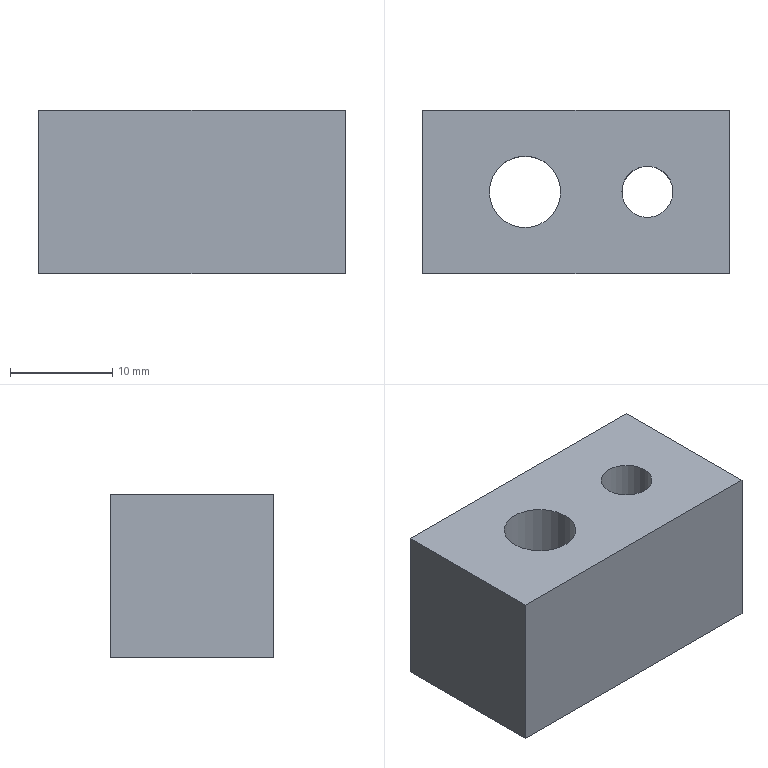Part | STEP file | 1_id1558_x_t | 1 solid | 12 faces | box 30 x 16 x 16 mm | volume 6176 mm3 | plane 7 | cylinder 4 | cone 1 | commonest cylinder face diameters 7 x2 5 x1 11 x1
STEP:
#1=CARTESIAN_POINT('',(0.,0.,0.));
#2=DIRECTION('',(0.,0.,1.));
#3=DIRECTION('',(1.,0.,0.));
#4=AXIS2_PLACEMENT_3D('',#1,#2,#3);
#5=CARTESIAN_POINT('',(359.525,145.5,108.11));
#6=VERTEX_POINT('',#5);
#7=CARTESIAN_POINT('',(357.025,145.5,108.11));
#8=DIRECTION('',(0.,0.,-1.));
#9=DIRECTION('',(1.,0.,0.));
#10=AXIS2_PLACEMENT_3D('',#7,#8,#9);
#11=CIRCLE('',#10,2.5);
#12=CARTESIAN_POINT('',(357.025,145.5,76.11));
#13=DIRECTION('',(0.,0.,1.));
#14=DIRECTION('',(1.,0.,0.));
#15=AXIS2_PLACEMENT_3D('',#12,#13,#14);
#16=CYLINDRICAL_SURFACE('',#15,2.5);
#17=CARTESIAN_POINT('',(6.283,32.));
#18=DIRECTION('',(-1.,0.));
#19=VECTOR('',#18,1.);
#20=LINE('',#17,#19);
#21=(GEOMETRIC_REPRESENTATION_CONTEXT(2)PARAMETRIC_REPRESENTATION_CONTEXT()REPRESENTATION_CONTEXT('',''));
#22=DEFINITIONAL_REPRESENTATION('',(#20),#21);
#23=PCURVE('',#16,#22);
#24=CARTESIAN_POINT('',(335.025,137.5,108.11));
#25=DIRECTION('',(0.,0.,-1.));
#26=DIRECTION('',(-1.,0.,0.));
#27=AXIS2_PLACEMENT_3D('',#24,#25,#26);
#28=PLANE('',#27);
#29=CARTESIAN_POINT('',(-22.,8.));
#30=DIRECTION('',(-1.,0.));
#31=AXIS2_PLACEMENT_2D('',#29,#30);
#32=CIRCLE('',#31,2.5);
#33=(GEOMETRIC_REPRESENTATION_CONTEXT(2)PARAMETRIC_REPRESENTATION_CONTEXT()REPRESENTATION_CONTEXT('',''));
#34=DEFINITIONAL_REPRESENTATION('',(#32),#33);
#35=PCURVE('',#28,#34);
#36=SURFACE_CURVE('',#11,(#23,#35),.PCURVE_S1.);
#37=EDGE_CURVE('',#6,#6,#36,.T.);
#38=ORIENTED_EDGE('',*,*,#37,.T.);
#39=CARTESIAN_POINT('',(359.525,145.5,99.11));
#40=VERTEX_POINT('',#39);
#41=CARTESIAN_POINT('',(359.525,145.5,99.11));
#42=CARTESIAN_POINT('',(359.525,145.5,108.11));
#43=B_SPLINE_CURVE_WITH_KNOTS('',1,(#41,#42),.UNSPECIFIED.,.F.,.F.,(2,2),(23.,32.),.PIECEWISE_BEZIER_KNOTS.);
#44=CARTESIAN_POINT('',(0.,0.));
#45=DIRECTION('',(0.,1.));
#46=VECTOR('',#45,1.);
#47=LINE('',#44,#46);
#48=(GEOMETRIC_REPRESENTATION_CONTEXT(2)PARAMETRIC_REPRESENTATION_CONTEXT()REPRESENTATION_CONTEXT('',''));
#49=DEFINITIONAL_REPRESENTATION('',(#47),#48);
#50=PCURVE('',#16,#49);
#51=CARTESIAN_POINT('',(6.283,0.));
#52=DIRECTION('',(0.,1.));
#53=VECTOR('',#52,1.);
#54=LINE('',#51,#53);
#55=(GEOMETRIC_REPRESENTATION_CONTEXT(2)PARAMETRIC_REPRESENTATION_CONTEXT()REPRESENTATION_CONTEXT('',''));
#56=DEFINITIONAL_REPRESENTATION('',(#54),#55);
#57=PCURVE('',#16,#56);
#58=SEAM_CURVE('',#43,(#50,#57),.PCURVE_S1.);
#59=EDGE_CURVE('',#40,#6,#58,.T.);
#60=ORIENTED_EDGE('',*,*,#59,.F.);
#61=CARTESIAN_POINT('',(354.525,145.5,99.11));
#62=VERTEX_POINT('',#61);
#63=CARTESIAN_POINT('',(357.025,145.5,99.11));
#64=DIRECTION('',(0.,0.,1.));
#65=DIRECTION('',(-1.,0.,0.));
#66=AXIS2_PLACEMENT_3D('',#63,#64,#65);
#67=CIRCLE('',#66,2.5);
#68=CARTESIAN_POINT('',(-3.142,23.));
#69=DIRECTION('',(1.,0.));
#70=VECTOR('',#69,1.);
#71=LINE('',#68,#70);
#72=(GEOMETRIC_REPRESENTATION_CONTEXT(2)PARAMETRIC_REPRESENTATION_CONTEXT()REPRESENTATION_CONTEXT('',''));
#73=DEFINITIONAL_REPRESENTATION('',(#71),#72);
#74=PCURVE('',#16,#73);
#75=CARTESIAN_POINT('',(357.025,145.5,98.61));
#76=DIRECTION('',(0.,0.,-1.));
#77=DIRECTION('',(-1.,0.,0.));
#78=AXIS2_PLACEMENT_3D('',#75,#76,#77);
#79=CONICAL_SURFACE('',#78,3.,0.7854);
#80=CARTESIAN_POINT('',(12.566,-0.5));
#81=DIRECTION('',(-1.,0.));
#82=VECTOR('',#81,1.);
#83=LINE('',#80,#82);
#84=(GEOMETRIC_REPRESENTATION_CONTEXT(2)PARAMETRIC_REPRESENTATION_CONTEXT()REPRESENTATION_CONTEXT('',''));
#85=DEFINITIONAL_REPRESENTATION('',(#83),#84);
#86=PCURVE('',#79,#85);
#87=SURFACE_CURVE('',#67,(#74,#86),.PCURVE_S1.);
#88=EDGE_CURVE('',#40,#62,#87,.T.);
#89=ORIENTED_EDGE('',*,*,#88,.T.);
#90=CARTESIAN_POINT('',(357.025,145.5,99.11));
#91=DIRECTION('',(0.,0.,1.));
#92=DIRECTION('',(-1.,0.,0.));
#93=AXIS2_PLACEMENT_3D('',#90,#91,#92);
#94=CIRCLE('',#93,2.5);
#95=CARTESIAN_POINT('',(3.142,23.));
#96=DIRECTION('',(1.,0.));
#97=VECTOR('',#96,1.);
#98=LINE('',#95,#97);
#99=(GEOMETRIC_REPRESENTATION_CONTEXT(2)PARAMETRIC_REPRESENTATION_CONTEXT()REPRESENTATION_CONTEXT('',''));
#100=DEFINITIONAL_REPRESENTATION('',(#98),#99);
#101=PCURVE('',#16,#100);
#102=CARTESIAN_POINT('',(6.283,-0.5));
#103=DIRECTION('',(-1.,0.));
#104=VECTOR('',#103,1.);
#105=LINE('',#102,#104);
#106=(GEOMETRIC_REPRESENTATION_CONTEXT(2)PARAMETRIC_REPRESENTATION_CONTEXT()REPRESENTATION_CONTEXT('',''));
#107=DEFINITIONAL_REPRESENTATION('',(#105),#106);
#108=PCURVE('',#79,#107);
#109=SURFACE_CURVE('',#94,(#101,#108),.PCURVE_S1.);
#110=EDGE_CURVE('',#62,#40,#109,.T.);
#111=ORIENTED_EDGE('',*,*,#110,.T.);
#112=ORIENTED_EDGE('',*,*,#59,.T.);
#113=EDGE_LOOP('',(#38,#60,#89,#111,#112));
#114=FACE_BOUND('',#113,.F.);
#115=ADVANCED_FACE('',(#114),#16,.F.);
#116=CARTESIAN_POINT('',(360.525,145.5,98.11));
#117=VERTEX_POINT('',#116);
#118=CARTESIAN_POINT('',(353.525,145.5,98.11));
#119=VERTEX_POINT('',#118);
#120=CARTESIAN_POINT('',(357.025,145.5,98.11));
#121=DIRECTION('',(0.,0.,-1.));
#122=DIRECTION('',(1.,0.,0.));
#123=AXIS2_PLACEMENT_3D('',#120,#121,#122);
#124=CIRCLE('',#123,3.5);
#125=CARTESIAN_POINT('',(3.142,0.5));
#126=DIRECTION('',(1.,0.));
#127=VECTOR('',#126,1.);
#128=LINE('',#125,#127);
#129=(GEOMETRIC_REPRESENTATION_CONTEXT(2)PARAMETRIC_REPRESENTATION_CONTEXT()REPRESENTATION_CONTEXT('',''));
#130=DEFINITIONAL_REPRESENTATION('',(#128),#129);
#131=PCURVE('',#79,#130);
#132=CARTESIAN_POINT('',(357.025,145.5,100.11));
#133=DIRECTION('',(0.,0.,-1.));
#134=DIRECTION('',(-1.,0.,0.));
#135=AXIS2_PLACEMENT_3D('',#132,#133,#134);
#136=CYLINDRICAL_SURFACE('',#135,3.5);
#137=CARTESIAN_POINT('',(3.142,2.));
#138=DIRECTION('',(1.,0.));
#139=VECTOR('',#138,1.);
#140=LINE('',#137,#139);
#141=(GEOMETRIC_REPRESENTATION_CONTEXT(2)PARAMETRIC_REPRESENTATION_CONTEXT()REPRESENTATION_CONTEXT('',''));
#142=DEFINITIONAL_REPRESENTATION('',(#140),#141);
#143=PCURVE('',#136,#142);
#144=SURFACE_CURVE('',#124,(#131,#143),.PCURVE_S1.);
#145=EDGE_CURVE('',#117,#119,#144,.T.);
#146=ORIENTED_EDGE('',*,*,#145,.F.);
#147=CARTESIAN_POINT('',(359.525,145.5,99.11));
#148=CARTESIAN_POINT('',(360.525,145.5,98.11));
#149=B_SPLINE_CURVE_WITH_KNOTS('',1,(#147,#148),.UNSPECIFIED.,.F.,.F.,(2,2),(-0.7071,0.7071),.PIECEWISE_BEZIER_KNOTS.);
#150=CARTESIAN_POINT('',(3.142,0.));
#151=DIRECTION('',(0.,1.));
#152=VECTOR('',#151,1.);
#153=LINE('',#150,#152);
#154=(GEOMETRIC_REPRESENTATION_CONTEXT(2)PARAMETRIC_REPRESENTATION_CONTEXT()REPRESENTATION_CONTEXT('',''));
#155=DEFINITIONAL_REPRESENTATION('',(#153),#154);
#156=PCURVE('',#79,#155);
#157=CARTESIAN_POINT('',(9.425,0.));
#158=DIRECTION('',(0.,1.));
#159=VECTOR('',#158,1.);
#160=LINE('',#157,#159);
#161=(GEOMETRIC_REPRESENTATION_CONTEXT(2)PARAMETRIC_REPRESENTATION_CONTEXT()REPRESENTATION_CONTEXT('',''));
#162=DEFINITIONAL_REPRESENTATION('',(#160),#161);
#163=PCURVE('',#79,#162);
#164=SEAM_CURVE('',#149,(#156,#163),.PCURVE_S1.);
#165=EDGE_CURVE('',#40,#117,#164,.T.);
#166=ORIENTED_EDGE('',*,*,#165,.F.);
#167=ORIENTED_EDGE('',*,*,#110,.F.);
#168=ORIENTED_EDGE('',*,*,#88,.F.);
#169=ORIENTED_EDGE('',*,*,#165,.T.);
#170=CARTESIAN_POINT('',(357.025,145.5,98.11));
#171=DIRECTION('',(0.,0.,-1.));
#172=DIRECTION('',(1.,0.,0.));
#173=AXIS2_PLACEMENT_3D('',#170,#171,#172);
#174=CIRCLE('',#173,3.5);
#175=CARTESIAN_POINT('',(3.142,0.5));
#176=DIRECTION('',(1.,0.));
#177=VECTOR('',#176,1.);
#178=LINE('',#175,#177);
#179=(GEOMETRIC_REPRESENTATION_CONTEXT(2)PARAMETRIC_REPRESENTATION_CONTEXT()REPRESENTATION_CONTEXT('',''));
#180=DEFINITIONAL_REPRESENTATION('',(#178),#179);
#181=PCURVE('',#79,#180);
#182=CARTESIAN_POINT('',(-3.142,2.));
#183=DIRECTION('',(1.,0.));
#184=VECTOR('',#183,1.);
#185=LINE('',#182,#184);
#186=(GEOMETRIC_REPRESENTATION_CONTEXT(2)PARAMETRIC_REPRESENTATION_CONTEXT()REPRESENTATION_CONTEXT('',''));
#187=DEFINITIONAL_REPRESENTATION('',(#185),#186);
#188=PCURVE('',#136,#187);
#189=SURFACE_CURVE('',#174,(#181,#188),.PCURVE_S1.);
#190=EDGE_CURVE('',#119,#117,#189,.T.);
#191=ORIENTED_EDGE('',*,*,#190,.F.);
#192=EDGE_LOOP('',(#146,#166,#167,#168,#169,#191));
#193=FACE_BOUND('',#192,.F.);
#194=ADVANCED_FACE('',(#193),#79,.F.);
#195=CARTESIAN_POINT('',(353.525,145.5,92.11));
#196=VERTEX_POINT('',#195);
#197=CARTESIAN_POINT('',(357.025,145.5,92.11));
#198=DIRECTION('',(0.,0.,1.));
#199=DIRECTION('',(-1.,0.,0.));
#200=AXIS2_PLACEMENT_3D('',#197,#198,#199);
#201=CIRCLE('',#200,3.5);
#202=CARTESIAN_POINT('',(6.283,8.));
#203=DIRECTION('',(-1.,0.));
#204=VECTOR('',#203,1.);
#205=LINE('',#202,#204);
#206=(GEOMETRIC_REPRESENTATION_CONTEXT(2)PARAMETRIC_REPRESENTATION_CONTEXT()REPRESENTATION_CONTEXT('',''));
#207=DEFINITIONAL_REPRESENTATION('',(#205),#206);
#208=PCURVE('',#136,#207);
#209=CARTESIAN_POINT('',(335.025,137.5,92.11));
#210=DIRECTION('',(0.,0.,-1.));
#211=DIRECTION('',(-1.,0.,0.));
#212=AXIS2_PLACEMENT_3D('',#209,#210,#211);
#213=PLANE('',#212);
#214=CARTESIAN_POINT('',(-18.5,8.));
#215=CARTESIAN_POINT('',(-18.5,1.938));
#216=CARTESIAN_POINT('',(-23.75,4.969));
#217=CARTESIAN_POINT('',(-29.,8.));
#218=CARTESIAN_POINT('',(-23.75,11.031));
#219=CARTESIAN_POINT('',(-18.5,14.062));
#220=CARTESIAN_POINT('',(-18.5,8.));
#221=(BOUNDED_CURVE()B_SPLINE_CURVE(2,(#214,#215,#216,#217,#218,#219,#220),.UNSPECIFIED.,.T.,.F.)B_SPLINE_CURVE_WITH_KNOTS((1,2,2,2,2,1),(-2.094,0.,2.094,4.189,6.283,8.378),.UNSPECIFIED.)CURVE()GEOMETRIC_REPRESENTATION_ITEM()RATIONAL_B_SPLINE_CURVE((1.,0.5,1.,0.5,1.,0.5,1.))REPRESENTATION_ITEM(''));
#222=(GEOMETRIC_REPRESENTATION_CONTEXT(2)PARAMETRIC_REPRESENTATION_CONTEXT()REPRESENTATION_CONTEXT('',''));
#223=DEFINITIONAL_REPRESENTATION('',(#221),#222);
#224=PCURVE('',#213,#223);
#225=SURFACE_CURVE('',#201,(#208,#224),.PCURVE_S1.);
#226=EDGE_CURVE('',#196,#196,#225,.T.);
#227=ORIENTED_EDGE('',*,*,#226,.T.);
#228=CARTESIAN_POINT('',(353.525,145.5,98.11));
#229=CARTESIAN_POINT('',(353.525,145.5,92.11));
#230=B_SPLINE_CURVE_WITH_KNOTS('',1,(#228,#229),.UNSPECIFIED.,.F.,.F.,(2,2),(2.,8.),.PIECEWISE_BEZIER_KNOTS.);
#231=CARTESIAN_POINT('',(0.,0.));
#232=DIRECTION('',(0.,1.));
#233=VECTOR('',#232,1.);
#234=LINE('',#231,#233);
#235=(GEOMETRIC_REPRESENTATION_CONTEXT(2)PARAMETRIC_REPRESENTATION_CONTEXT()REPRESENTATION_CONTEXT('',''));
#236=DEFINITIONAL_REPRESENTATION('',(#234),#235);
#237=PCURVE('',#136,#236);
#238=CARTESIAN_POINT('',(6.283,0.));
#239=DIRECTION('',(0.,1.));
#240=VECTOR('',#239,1.);
#241=LINE('',#238,#240);
#242=(GEOMETRIC_REPRESENTATION_CONTEXT(2)PARAMETRIC_REPRESENTATION_CONTEXT()REPRESENTATION_CONTEXT('',''));
#243=DEFINITIONAL_REPRESENTATION('',(#241),#242);
#244=PCURVE('',#136,#243);
#245=SEAM_CURVE('',#230,(#237,#244),.PCURVE_S1.);
#246=EDGE_CURVE('',#119,#196,#245,.T.);
#247=ORIENTED_EDGE('',*,*,#246,.F.);
#248=ORIENTED_EDGE('',*,*,#190,.T.);
#249=ORIENTED_EDGE('',*,*,#145,.T.);
#250=ORIENTED_EDGE('',*,*,#246,.T.);
#251=EDGE_LOOP('',(#227,#247,#248,#249,#250));
#252=FACE_BOUND('',#251,.F.);
#253=ADVANCED_FACE('',(#252),#136,.F.);
#254=CARTESIAN_POINT('',(335.025,153.5,108.11));
#255=VERTEX_POINT('',#254);
#256=CARTESIAN_POINT('',(335.025,137.5,108.11));
#257=VERTEX_POINT('',#256);
#258=CARTESIAN_POINT('',(335.025,153.5,108.11));
#259=DIRECTION('',(0.,-1.,0.));
#260=VECTOR('',#259,1.);
#261=LINE('',#258,#260);
#262=CARTESIAN_POINT('',(0.,16.));
#263=DIRECTION('',(0.,-1.));
#264=VECTOR('',#263,1.);
#265=LINE('',#262,#264);
#266=(GEOMETRIC_REPRESENTATION_CONTEXT(2)PARAMETRIC_REPRESENTATION_CONTEXT()REPRESENTATION_CONTEXT('',''));
#267=DEFINITIONAL_REPRESENTATION('',(#265),#266);
#268=PCURVE('',#28,#267);
#269=CARTESIAN_POINT('',(335.025,137.5,92.11));
#270=DIRECTION('',(1.,0.,0.));
#271=DIRECTION('',(0.,0.,-1.));
#272=AXIS2_PLACEMENT_3D('',#269,#270,#271);
#273=PLANE('',#272);
#274=CARTESIAN_POINT('',(-16.,16.));
#275=DIRECTION('',(0.,-1.));
#276=VECTOR('',#275,1.);
#277=LINE('',#274,#276);
#278=(GEOMETRIC_REPRESENTATION_CONTEXT(2)PARAMETRIC_REPRESENTATION_CONTEXT()REPRESENTATION_CONTEXT('',''));
#279=DEFINITIONAL_REPRESENTATION('',(#277),#278);
#280=PCURVE('',#273,#279);
#281=SURFACE_CURVE('',#261,(#268,#280),.PCURVE_S1.);
#282=EDGE_CURVE('',#255,#257,#281,.T.);
#283=ORIENTED_EDGE('',*,*,#282,.T.);
#284=CARTESIAN_POINT('',(365.025,137.5,108.11));
#285=VERTEX_POINT('',#284);
#286=CARTESIAN_POINT('',(335.025,137.5,108.11));
#287=DIRECTION('',(1.,0.,0.));
#288=VECTOR('',#287,1.);
#289=LINE('',#286,#288);
#290=CARTESIAN_POINT('',(0.,0.));
#291=DIRECTION('',(-1.,0.));
#292=VECTOR('',#291,1.);
#293=LINE('',#290,#292);
#294=(GEOMETRIC_REPRESENTATION_CONTEXT(2)PARAMETRIC_REPRESENTATION_CONTEXT()REPRESENTATION_CONTEXT('',''));
#295=DEFINITIONAL_REPRESENTATION('',(#293),#294);
#296=PCURVE('',#28,#295);
#297=CARTESIAN_POINT('',(365.025,137.5,92.11));
#298=DIRECTION('',(0.,1.,0.));
#299=DIRECTION('',(0.,0.,-1.));
#300=AXIS2_PLACEMENT_3D('',#297,#298,#299);
#301=PLANE('',#300);
#302=CARTESIAN_POINT('',(-16.,30.));
#303=DIRECTION('',(0.,-1.));
#304=VECTOR('',#303,1.);
#305=LINE('',#302,#304);
#306=(GEOMETRIC_REPRESENTATION_CONTEXT(2)PARAMETRIC_REPRESENTATION_CONTEXT()REPRESENTATION_CONTEXT('',''));
#307=DEFINITIONAL_REPRESENTATION('',(#305),#306);
#308=PCURVE('',#301,#307);
#309=SURFACE_CURVE('',#289,(#296,#308),.PCURVE_S1.);
#310=EDGE_CURVE('',#257,#285,#309,.T.);
#311=ORIENTED_EDGE('',*,*,#310,.T.);
#312=CARTESIAN_POINT('',(365.025,153.5,108.11));
#313=VERTEX_POINT('',#312);
#314=CARTESIAN_POINT('',(365.025,137.5,108.11));
#315=DIRECTION('',(0.,1.,0.));
#316=VECTOR('',#315,1.);
#317=LINE('',#314,#316);
#318=CARTESIAN_POINT('',(-30.,0.));
#319=DIRECTION('',(0.,1.));
#320=VECTOR('',#319,1.);
#321=LINE('',#318,#320);
#322=(GEOMETRIC_REPRESENTATION_CONTEXT(2)PARAMETRIC_REPRESENTATION_CONTEXT()REPRESENTATION_CONTEXT('',''));
#323=DEFINITIONAL_REPRESENTATION('',(#321),#322);
#324=PCURVE('',#28,#323);
#325=CARTESIAN_POINT('',(365.025,153.5,92.11));
#326=DIRECTION('',(-1.,0.,0.));
#327=DIRECTION('',(0.,0.,1.));
#328=AXIS2_PLACEMENT_3D('',#325,#326,#327);
#329=PLANE('',#328);
#330=CARTESIAN_POINT('',(16.,-16.));
#331=DIRECTION('',(0.,1.));
#332=VECTOR('',#331,1.);
#333=LINE('',#330,#332);
#334=(GEOMETRIC_REPRESENTATION_CONTEXT(2)PARAMETRIC_REPRESENTATION_CONTEXT()REPRESENTATION_CONTEXT('',''));
#335=DEFINITIONAL_REPRESENTATION('',(#333),#334);
#336=PCURVE('',#329,#335);
#337=SURFACE_CURVE('',#317,(#324,#336),.PCURVE_S1.);
#338=EDGE_CURVE('',#285,#313,#337,.T.);
#339=ORIENTED_EDGE('',*,*,#338,.T.);
#340=CARTESIAN_POINT('',(365.025,153.5,108.11));
#341=DIRECTION('',(-1.,0.,0.));
#342=VECTOR('',#341,1.);
#343=LINE('',#340,#342);
#344=CARTESIAN_POINT('',(-30.,16.));
#345=DIRECTION('',(1.,0.));
#346=VECTOR('',#345,1.);
#347=LINE('',#344,#346);
#348=(GEOMETRIC_REPRESENTATION_CONTEXT(2)PARAMETRIC_REPRESENTATION_CONTEXT()REPRESENTATION_CONTEXT('',''));
#349=DEFINITIONAL_REPRESENTATION('',(#347),#348);
#350=PCURVE('',#28,#349);
#351=CARTESIAN_POINT('',(335.025,153.5,92.11));
#352=DIRECTION('',(0.,-1.,0.));
#353=DIRECTION('',(0.,0.,1.));
#354=AXIS2_PLACEMENT_3D('',#351,#352,#353);
#355=PLANE('',#354);
#356=CARTESIAN_POINT('',(16.,-30.));
#357=DIRECTION('',(0.,1.));
#358=VECTOR('',#357,1.);
#359=LINE('',#356,#358);
#360=(GEOMETRIC_REPRESENTATION_CONTEXT(2)PARAMETRIC_REPRESENTATION_CONTEXT()REPRESENTATION_CONTEXT('',''));
#361=DEFINITIONAL_REPRESENTATION('',(#359),#360);
#362=PCURVE('',#355,#361);
#363=SURFACE_CURVE('',#343,(#350,#362),.PCURVE_S1.);
#364=EDGE_CURVE('',#313,#255,#363,.T.);
#365=ORIENTED_EDGE('',*,*,#364,.T.);
#366=EDGE_LOOP('',(#283,#311,#339,#365));
#367=FACE_BOUND('',#366,.T.);
#368=ORIENTED_EDGE('',*,*,#37,.T.);
#369=EDGE_LOOP('',(#368));
#370=FACE_BOUND('',#369,.T.);
#371=CARTESIAN_POINT('',(348.525,145.5,108.11));
#372=VERTEX_POINT('',#371);
#373=CARTESIAN_POINT('',(345.025,145.5,108.11));
#374=DIRECTION('',(0.,0.,-1.));
#375=DIRECTION('',(1.,0.,0.));
#376=AXIS2_PLACEMENT_3D('',#373,#374,#375);
#377=CIRCLE('',#376,3.5);
#378=CARTESIAN_POINT('',(-10.,8.));
#379=DIRECTION('',(-1.,0.));
#380=AXIS2_PLACEMENT_2D('',#378,#379);
#381=CIRCLE('',#380,3.5);
#382=(GEOMETRIC_REPRESENTATION_CONTEXT(2)PARAMETRIC_REPRESENTATION_CONTEXT()REPRESENTATION_CONTEXT('',''));
#383=DEFINITIONAL_REPRESENTATION('',(#381),#382);
#384=PCURVE('',#28,#383);
#385=CARTESIAN_POINT('',(345.025,145.5,76.11));
#386=DIRECTION('',(0.,0.,1.));
#387=DIRECTION('',(1.,0.,0.));
#388=AXIS2_PLACEMENT_3D('',#385,#386,#387);
#389=CYLINDRICAL_SURFACE('',#388,3.5);
#390=CARTESIAN_POINT('',(6.283,32.));
#391=DIRECTION('',(-1.,0.));
#392=VECTOR('',#391,1.);
#393=LINE('',#390,#392);
#394=(GEOMETRIC_REPRESENTATION_CONTEXT(2)PARAMETRIC_REPRESENTATION_CONTEXT()REPRESENTATION_CONTEXT('',''));
#395=DEFINITIONAL_REPRESENTATION('',(#393),#394);
#396=PCURVE('',#389,#395);
#397=SURFACE_CURVE('',#377,(#384,#396),.PCURVE_S1.);
#398=EDGE_CURVE('',#372,#372,#397,.T.);
#399=ORIENTED_EDGE('',*,*,#398,.T.);
#400=EDGE_LOOP('',(#399));
#401=FACE_BOUND('',#400,.T.);
#402=ADVANCED_FACE('',(#367,#370,#401),#28,.F.);
#403=CARTESIAN_POINT('',(335.025,153.5,92.11));
#404=VERTEX_POINT('',#403);
#405=CARTESIAN_POINT('',(335.025,153.5,92.11));
#406=DIRECTION('',(0.,0.,1.));
#407=VECTOR('',#406,1.);
#408=LINE('',#405,#407);
#409=CARTESIAN_POINT('',(0.,0.));
#410=DIRECTION('',(1.,0.));
#411=VECTOR('',#410,1.);
#412=LINE('',#409,#411);
#413=(GEOMETRIC_REPRESENTATION_CONTEXT(2)PARAMETRIC_REPRESENTATION_CONTEXT()REPRESENTATION_CONTEXT('',''));
#414=DEFINITIONAL_REPRESENTATION('',(#412),#413);
#415=PCURVE('',#355,#414);
#416=CARTESIAN_POINT('',(0.,16.));
#417=DIRECTION('',(-1.,0.));
#418=VECTOR('',#417,1.);
#419=LINE('',#416,#418);
#420=(GEOMETRIC_REPRESENTATION_CONTEXT(2)PARAMETRIC_REPRESENTATION_CONTEXT()REPRESENTATION_CONTEXT('',''));
#421=DEFINITIONAL_REPRESENTATION('',(#419),#420);
#422=PCURVE('',#273,#421);
#423=SURFACE_CURVE('',#408,(#415,#422),.PCURVE_S1.);
#424=EDGE_CURVE('',#404,#255,#423,.T.);
#425=ORIENTED_EDGE('',*,*,#424,.T.);
#426=ORIENTED_EDGE('',*,*,#364,.F.);
#427=CARTESIAN_POINT('',(365.025,153.5,92.11));
#428=VERTEX_POINT('',#427);
#429=CARTESIAN_POINT('',(365.025,153.5,92.11));
#430=DIRECTION('',(0.,0.,1.));
#431=VECTOR('',#430,1.);
#432=LINE('',#429,#431);
#433=CARTESIAN_POINT('',(0.,-30.));
#434=DIRECTION('',(1.,0.));
#435=VECTOR('',#434,1.);
#436=LINE('',#433,#435);
#437=(GEOMETRIC_REPRESENTATION_CONTEXT(2)PARAMETRIC_REPRESENTATION_CONTEXT()REPRESENTATION_CONTEXT('',''));
#438=DEFINITIONAL_REPRESENTATION('',(#436),#437);
#439=PCURVE('',#355,#438);
#440=CARTESIAN_POINT('',(0.,0.));
#441=DIRECTION('',(1.,0.));
#442=VECTOR('',#441,1.);
#443=LINE('',#440,#442);
#444=(GEOMETRIC_REPRESENTATION_CONTEXT(2)PARAMETRIC_REPRESENTATION_CONTEXT()REPRESENTATION_CONTEXT('',''));
#445=DEFINITIONAL_REPRESENTATION('',(#443),#444);
#446=PCURVE('',#329,#445);
#447=SURFACE_CURVE('',#432,(#439,#446),.PCURVE_S1.);
#448=EDGE_CURVE('',#428,#313,#447,.T.);
#449=ORIENTED_EDGE('',*,*,#448,.F.);
#450=CARTESIAN_POINT('',(365.025,153.5,92.11));
#451=DIRECTION('',(-1.,0.,0.));
#452=VECTOR('',#451,1.);
#453=LINE('',#450,#452);
#454=CARTESIAN_POINT('',(0.,-30.));
#455=DIRECTION('',(0.,1.));
#456=VECTOR('',#455,1.);
#457=LINE('',#454,#456);
#458=(GEOMETRIC_REPRESENTATION_CONTEXT(2)PARAMETRIC_REPRESENTATION_CONTEXT()REPRESENTATION_CONTEXT('',''));
#459=DEFINITIONAL_REPRESENTATION('',(#457),#458);
#460=PCURVE('',#355,#459);
#461=CARTESIAN_POINT('',(-30.,16.));
#462=DIRECTION('',(1.,0.));
#463=VECTOR('',#462,1.);
#464=LINE('',#461,#463);
#465=(GEOMETRIC_REPRESENTATION_CONTEXT(2)PARAMETRIC_REPRESENTATION_CONTEXT()REPRESENTATION_CONTEXT('',''));
#466=DEFINITIONAL_REPRESENTATION('',(#464),#465);
#467=PCURVE('',#213,#466);
#468=SURFACE_CURVE('',#453,(#460,#467),.PCURVE_S1.);
#469=EDGE_CURVE('',#428,#404,#468,.T.);
#470=ORIENTED_EDGE('',*,*,#469,.T.);
#471=EDGE_LOOP('',(#425,#426,#449,#470));
#472=FACE_BOUND('',#471,.T.);
#473=ADVANCED_FACE('',(#472),#355,.F.);
#474=ORIENTED_EDGE('',*,*,#469,.F.);
#475=CARTESIAN_POINT('',(365.025,137.5,92.11));
#476=VERTEX_POINT('',#475);
#477=CARTESIAN_POINT('',(365.025,137.5,92.11));
#478=DIRECTION('',(0.,1.,0.));
#479=VECTOR('',#478,1.);
#480=LINE('',#477,#479);
#481=CARTESIAN_POINT('',(-30.,0.));
#482=DIRECTION('',(0.,1.));
#483=VECTOR('',#482,1.);
#484=LINE('',#481,#483);
#485=(GEOMETRIC_REPRESENTATION_CONTEXT(2)PARAMETRIC_REPRESENTATION_CONTEXT()REPRESENTATION_CONTEXT('',''));
#486=DEFINITIONAL_REPRESENTATION('',(#484),#485);
#487=PCURVE('',#213,#486);
#488=CARTESIAN_POINT('',(0.,-16.));
#489=DIRECTION('',(0.,1.));
#490=VECTOR('',#489,1.);
#491=LINE('',#488,#490);
#492=(GEOMETRIC_REPRESENTATION_CONTEXT(2)PARAMETRIC_REPRESENTATION_CONTEXT()REPRESENTATION_CONTEXT('',''));
#493=DEFINITIONAL_REPRESENTATION('',(#491),#492);
#494=PCURVE('',#329,#493);
#495=SURFACE_CURVE('',#480,(#487,#494),.PCURVE_S1.);
#496=EDGE_CURVE('',#476,#428,#495,.T.);
#497=ORIENTED_EDGE('',*,*,#496,.F.);
#498=CARTESIAN_POINT('',(335.025,137.5,92.11));
#499=VERTEX_POINT('',#498);
#500=CARTESIAN_POINT('',(335.025,137.5,92.11));
#501=DIRECTION('',(1.,0.,0.));
#502=VECTOR('',#501,1.);
#503=LINE('',#500,#502);
#504=CARTESIAN_POINT('',(0.,0.));
#505=DIRECTION('',(-1.,0.));
#506=VECTOR('',#505,1.);
#507=LINE('',#504,#506);
#508=(GEOMETRIC_REPRESENTATION_CONTEXT(2)PARAMETRIC_REPRESENTATION_CONTEXT()REPRESENTATION_CONTEXT('',''));
#509=DEFINITIONAL_REPRESENTATION('',(#507),#508);
#510=PCURVE('',#213,#509);
#511=CARTESIAN_POINT('',(0.,30.));
#512=DIRECTION('',(0.,-1.));
#513=VECTOR('',#512,1.);
#514=LINE('',#511,#513);
#515=(GEOMETRIC_REPRESENTATION_CONTEXT(2)PARAMETRIC_REPRESENTATION_CONTEXT()REPRESENTATION_CONTEXT('',''));
#516=DEFINITIONAL_REPRESENTATION('',(#514),#515);
#517=PCURVE('',#301,#516);
#518=SURFACE_CURVE('',#503,(#510,#517),.PCURVE_S1.);
#519=EDGE_CURVE('',#499,#476,#518,.T.);
#520=ORIENTED_EDGE('',*,*,#519,.F.);
#521=CARTESIAN_POINT('',(335.025,153.5,92.11));
#522=DIRECTION('',(0.,-1.,0.));
#523=VECTOR('',#522,1.);
#524=LINE('',#521,#523);
#525=CARTESIAN_POINT('',(0.,16.));
#526=DIRECTION('',(0.,-1.));
#527=VECTOR('',#526,1.);
#528=LINE('',#525,#527);
#529=(GEOMETRIC_REPRESENTATION_CONTEXT(2)PARAMETRIC_REPRESENTATION_CONTEXT()REPRESENTATION_CONTEXT('',''));
#530=DEFINITIONAL_REPRESENTATION('',(#528),#529);
#531=PCURVE('',#213,#530);
#532=CARTESIAN_POINT('',(0.,16.));
#533=DIRECTION('',(0.,-1.));
#534=VECTOR('',#533,1.);
#535=LINE('',#532,#534);
#536=(GEOMETRIC_REPRESENTATION_CONTEXT(2)PARAMETRIC_REPRESENTATION_CONTEXT()REPRESENTATION_CONTEXT('',''));
#537=DEFINITIONAL_REPRESENTATION('',(#535),#536);
#538=PCURVE('',#273,#537);
#539=SURFACE_CURVE('',#524,(#531,#538),.PCURVE_S1.);
#540=EDGE_CURVE('',#404,#499,#539,.T.);
#541=ORIENTED_EDGE('',*,*,#540,.F.);
#542=EDGE_LOOP('',(#474,#497,#520,#541));
#543=FACE_BOUND('',#542,.T.);
#544=ORIENTED_EDGE('',*,*,#226,.T.);
#545=EDGE_LOOP('',(#544));
#546=FACE_BOUND('',#545,.T.);
#547=CARTESIAN_POINT('',(350.525,145.5,92.11));
#548=VERTEX_POINT('',#547);
#549=CARTESIAN_POINT('',(339.525,145.5,92.11));
#550=VERTEX_POINT('',#549);
#551=CARTESIAN_POINT('',(345.025,145.5,92.11));
#552=DIRECTION('',(0.,0.,1.));
#553=DIRECTION('',(1.,0.,0.));
#554=AXIS2_PLACEMENT_3D('',#551,#552,#553);
#555=CIRCLE('',#554,5.5);
#556=CARTESIAN_POINT('',(-15.5,8.));
#557=CARTESIAN_POINT('',(-15.5,17.526));
#558=CARTESIAN_POINT('',(-7.25,12.763));
#559=CARTESIAN_POINT('',(1.,8.));
#560=CARTESIAN_POINT('',(-7.25,3.237));
#561=CARTESIAN_POINT('',(-15.5,-1.526));
#562=CARTESIAN_POINT('',(-15.5,8.));
#563=(BOUNDED_CURVE()B_SPLINE_CURVE(2,(#556,#557,#558,#559,#560,#561,#562),.UNSPECIFIED.,.T.,.F.)B_SPLINE_CURVE_WITH_KNOTS((1,2,2,2,2,1),(-2.094,0.,2.094,4.189,6.283,8.378),.UNSPECIFIED.)CURVE()GEOMETRIC_REPRESENTATION_ITEM()RATIONAL_B_SPLINE_CURVE((1.,0.5,1.,0.5,1.,0.5,1.))REPRESENTATION_ITEM(''));
#564=(GEOMETRIC_REPRESENTATION_CONTEXT(2)PARAMETRIC_REPRESENTATION_CONTEXT()REPRESENTATION_CONTEXT('',''));
#565=DEFINITIONAL_REPRESENTATION('',(#563),#564);
#566=PCURVE('',#213,#565);
#567=CARTESIAN_POINT('',(345.025,145.5,100.11));
#568=DIRECTION('',(0.,0.,-1.));
#569=DIRECTION('',(-1.,0.,0.));
#570=AXIS2_PLACEMENT_3D('',#567,#568,#569);
#571=CYLINDRICAL_SURFACE('',#570,5.5);
#572=CARTESIAN_POINT('',(3.142,8.));
#573=DIRECTION('',(-1.,0.));
#574=VECTOR('',#573,1.);
#575=LINE('',#572,#574);
#576=(GEOMETRIC_REPRESENTATION_CONTEXT(2)PARAMETRIC_REPRESENTATION_CONTEXT()REPRESENTATION_CONTEXT('',''));
#577=DEFINITIONAL_REPRESENTATION('',(#575),#576);
#578=PCURVE('',#571,#577);
#579=SURFACE_CURVE('',#555,(#566,#578),.PCURVE_S1.);
#580=EDGE_CURVE('',#548,#550,#579,.T.);
#581=ORIENTED_EDGE('',*,*,#580,.T.);
#582=CARTESIAN_POINT('',(345.025,145.5,92.11));
#583=DIRECTION('',(0.,0.,1.));
#584=DIRECTION('',(1.,0.,0.));
#585=AXIS2_PLACEMENT_3D('',#582,#583,#584);
#586=CIRCLE('',#585,5.5);
#587=CARTESIAN_POINT('',(-15.5,8.));
#588=CARTESIAN_POINT('',(-15.5,17.526));
#589=CARTESIAN_POINT('',(-7.25,12.763));
#590=CARTESIAN_POINT('',(1.,8.));
#591=CARTESIAN_POINT('',(-7.25,3.237));
#592=CARTESIAN_POINT('',(-15.5,-1.526));
#593=CARTESIAN_POINT('',(-15.5,8.));
#594=(BOUNDED_CURVE()B_SPLINE_CURVE(2,(#587,#588,#589,#590,#591,#592,#593),.UNSPECIFIED.,.T.,.F.)B_SPLINE_CURVE_WITH_KNOTS((1,2,2,2,2,1),(-2.094,0.,2.094,4.189,6.283,8.378),.UNSPECIFIED.)CURVE()GEOMETRIC_REPRESENTATION_ITEM()RATIONAL_B_SPLINE_CURVE((1.,0.5,1.,0.5,1.,0.5,1.))REPRESENTATION_ITEM(''));
#595=(GEOMETRIC_REPRESENTATION_CONTEXT(2)PARAMETRIC_REPRESENTATION_CONTEXT()REPRESENTATION_CONTEXT('',''));
#596=DEFINITIONAL_REPRESENTATION('',(#594),#595);
#597=PCURVE('',#213,#596);
#598=CARTESIAN_POINT('',(9.425,8.));
#599=DIRECTION('',(-1.,0.));
#600=VECTOR('',#599,1.);
#601=LINE('',#598,#600);
#602=(GEOMETRIC_REPRESENTATION_CONTEXT(2)PARAMETRIC_REPRESENTATION_CONTEXT()REPRESENTATION_CONTEXT('',''));
#603=DEFINITIONAL_REPRESENTATION('',(#601),#602);
#604=PCURVE('',#571,#603);
#605=SURFACE_CURVE('',#586,(#597,#604),.PCURVE_S1.);
#606=EDGE_CURVE('',#550,#548,#605,.T.);
#607=ORIENTED_EDGE('',*,*,#606,.T.);
#608=EDGE_LOOP('',(#581,#607));
#609=FACE_BOUND('',#608,.T.);
#610=ADVANCED_FACE('',(#543,#546,#609),#213,.T.);
#611=ORIENTED_EDGE('',*,*,#580,.T.);
#612=CARTESIAN_POINT('',(339.525,145.5,100.11));
#613=VERTEX_POINT('',#612);
#614=CARTESIAN_POINT('',(339.525,145.5,100.11));
#615=CARTESIAN_POINT('',(339.525,145.5,92.11));
#616=B_SPLINE_CURVE_WITH_KNOTS('',1,(#614,#615),.UNSPECIFIED.,.F.,.F.,(2,2),(0.,8.),.PIECEWISE_BEZIER_KNOTS.);
#617=CARTESIAN_POINT('',(0.,0.));
#618=DIRECTION('',(0.,1.));
#619=VECTOR('',#618,1.);
#620=LINE('',#617,#619);
#621=(GEOMETRIC_REPRESENTATION_CONTEXT(2)PARAMETRIC_REPRESENTATION_CONTEXT()REPRESENTATION_CONTEXT('',''));
#622=DEFINITIONAL_REPRESENTATION('',(#620),#621);
#623=PCURVE('',#571,#622);
#624=CARTESIAN_POINT('',(6.283,0.));
#625=DIRECTION('',(0.,1.));
#626=VECTOR('',#625,1.);
#627=LINE('',#624,#626);
#628=(GEOMETRIC_REPRESENTATION_CONTEXT(2)PARAMETRIC_REPRESENTATION_CONTEXT()REPRESENTATION_CONTEXT('',''));
#629=DEFINITIONAL_REPRESENTATION('',(#627),#628);
#630=PCURVE('',#571,#629);
#631=SEAM_CURVE('',#616,(#623,#630),.PCURVE_S1.);
#632=EDGE_CURVE('',#613,#550,#631,.T.);
#633=ORIENTED_EDGE('',*,*,#632,.F.);
#634=CARTESIAN_POINT('',(345.025,145.5,100.11));
#635=DIRECTION('',(0.,0.,-1.));
#636=DIRECTION('',(-1.,0.,0.));
#637=AXIS2_PLACEMENT_3D('',#634,#635,#636);
#638=CIRCLE('',#637,5.5);
#639=CARTESIAN_POINT('',(0.,0.));
#640=DIRECTION('',(1.,0.));
#641=VECTOR('',#640,1.);
#642=LINE('',#639,#641);
#643=(GEOMETRIC_REPRESENTATION_CONTEXT(2)PARAMETRIC_REPRESENTATION_CONTEXT()REPRESENTATION_CONTEXT('',''));
#644=DEFINITIONAL_REPRESENTATION('',(#642),#643);
#645=PCURVE('',#571,#644);
#646=CARTESIAN_POINT('',(345.025,145.5,100.11));
#647=DIRECTION('',(0.,0.,-1.));
#648=DIRECTION('',(-1.,0.,0.));
#649=AXIS2_PLACEMENT_3D('',#646,#647,#648);
#650=PLANE('',#649);
#651=CARTESIAN_POINT('',(0.,0.));
#652=DIRECTION('',(1.,0.));
#653=AXIS2_PLACEMENT_2D('',#651,#652);
#654=CIRCLE('',#653,5.5);
#655=(GEOMETRIC_REPRESENTATION_CONTEXT(2)PARAMETRIC_REPRESENTATION_CONTEXT()REPRESENTATION_CONTEXT('',''));
#656=DEFINITIONAL_REPRESENTATION('',(#654),#655);
#657=PCURVE('',#650,#656);
#658=SURFACE_CURVE('',#638,(#645,#657),.PCURVE_S1.);
#659=EDGE_CURVE('',#613,#613,#658,.T.);
#660=ORIENTED_EDGE('',*,*,#659,.T.);
#661=ORIENTED_EDGE('',*,*,#632,.T.);
#662=ORIENTED_EDGE('',*,*,#606,.T.);
#663=EDGE_LOOP('',(#611,#633,#660,#661,#662));
#664=FACE_BOUND('',#663,.F.);
#665=ADVANCED_FACE('',(#664),#571,.F.);
#666=ORIENTED_EDGE('',*,*,#659,.T.);
#667=EDGE_LOOP('',(#666));
#668=FACE_BOUND('',#667,.T.);
#669=CARTESIAN_POINT('',(348.525,145.5,100.11));
#670=VERTEX_POINT('',#669);
#671=CARTESIAN_POINT('',(345.025,145.5,100.11));
#672=DIRECTION('',(0.,0.,1.));
#673=DIRECTION('',(1.,0.,0.));
#674=AXIS2_PLACEMENT_3D('',#671,#672,#673);
#675=CIRCLE('',#674,3.5);
#676=CARTESIAN_POINT('',(-3.5,0.));
#677=CARTESIAN_POINT('',(-3.5,6.062));
#678=CARTESIAN_POINT('',(1.75,3.031));
#679=CARTESIAN_POINT('',(7.,0.));
#680=CARTESIAN_POINT('',(1.75,-3.031));
#681=CARTESIAN_POINT('',(-3.5,-6.062));
#682=CARTESIAN_POINT('',(-3.5,0.));
#683=(BOUNDED_CURVE()B_SPLINE_CURVE(2,(#676,#677,#678,#679,#680,#681,#682),.UNSPECIFIED.,.T.,.F.)B_SPLINE_CURVE_WITH_KNOTS((1,2,2,2,2,1),(-2.094,0.,2.094,4.189,6.283,8.378),.UNSPECIFIED.)CURVE()GEOMETRIC_REPRESENTATION_ITEM()RATIONAL_B_SPLINE_CURVE((1.,0.5,1.,0.5,1.,0.5,1.))REPRESENTATION_ITEM(''));
#684=(GEOMETRIC_REPRESENTATION_CONTEXT(2)PARAMETRIC_REPRESENTATION_CONTEXT()REPRESENTATION_CONTEXT('',''));
#685=DEFINITIONAL_REPRESENTATION('',(#683),#684);
#686=PCURVE('',#650,#685);
#687=CARTESIAN_POINT('',(0.,24.));
#688=DIRECTION('',(1.,0.));
#689=VECTOR('',#688,1.);
#690=LINE('',#687,#689);
#691=(GEOMETRIC_REPRESENTATION_CONTEXT(2)PARAMETRIC_REPRESENTATION_CONTEXT()REPRESENTATION_CONTEXT('',''));
#692=DEFINITIONAL_REPRESENTATION('',(#690),#691);
#693=PCURVE('',#389,#692);
#694=SURFACE_CURVE('',#675,(#686,#693),.PCURVE_S1.);
#695=EDGE_CURVE('',#670,#670,#694,.T.);
#696=ORIENTED_EDGE('',*,*,#695,.T.);
#697=EDGE_LOOP('',(#696));
#698=FACE_BOUND('',#697,.T.);
#699=ADVANCED_FACE('',(#668,#698),#650,.T.);
#700=ORIENTED_EDGE('',*,*,#398,.T.);
#701=CARTESIAN_POINT('',(348.525,145.5,100.11));
#702=CARTESIAN_POINT('',(348.525,145.5,108.11));
#703=B_SPLINE_CURVE_WITH_KNOTS('',1,(#701,#702),.UNSPECIFIED.,.F.,.F.,(2,2),(24.,32.),.PIECEWISE_BEZIER_KNOTS.);
#704=CARTESIAN_POINT('',(0.,0.));
#705=DIRECTION('',(0.,1.));
#706=VECTOR('',#705,1.);
#707=LINE('',#704,#706);
#708=(GEOMETRIC_REPRESENTATION_CONTEXT(2)PARAMETRIC_REPRESENTATION_CONTEXT()REPRESENTATION_CONTEXT('',''));
#709=DEFINITIONAL_REPRESENTATION('',(#707),#708);
#710=PCURVE('',#389,#709);
#711=CARTESIAN_POINT('',(6.283,0.));
#712=DIRECTION('',(0.,1.));
#713=VECTOR('',#712,1.);
#714=LINE('',#711,#713);
#715=(GEOMETRIC_REPRESENTATION_CONTEXT(2)PARAMETRIC_REPRESENTATION_CONTEXT()REPRESENTATION_CONTEXT('',''));
#716=DEFINITIONAL_REPRESENTATION('',(#714),#715);
#717=PCURVE('',#389,#716);
#718=SEAM_CURVE('',#703,(#710,#717),.PCURVE_S1.);
#719=EDGE_CURVE('',#670,#372,#718,.T.);
#720=ORIENTED_EDGE('',*,*,#719,.F.);
#721=ORIENTED_EDGE('',*,*,#695,.T.);
#722=ORIENTED_EDGE('',*,*,#719,.T.);
#723=EDGE_LOOP('',(#700,#720,#721,#722));
#724=FACE_BOUND('',#723,.F.);
#725=ADVANCED_FACE('',(#724),#389,.F.);
#726=ORIENTED_EDGE('',*,*,#424,.F.);
#727=ORIENTED_EDGE('',*,*,#540,.T.);
#728=CARTESIAN_POINT('',(335.025,137.5,92.11));
#729=DIRECTION('',(0.,0.,1.));
#730=VECTOR('',#729,1.);
#731=LINE('',#728,#730);
#732=CARTESIAN_POINT('',(0.,0.));
#733=DIRECTION('',(-1.,0.));
#734=VECTOR('',#733,1.);
#735=LINE('',#732,#734);
#736=(GEOMETRIC_REPRESENTATION_CONTEXT(2)PARAMETRIC_REPRESENTATION_CONTEXT()REPRESENTATION_CONTEXT('',''));
#737=DEFINITIONAL_REPRESENTATION('',(#735),#736);
#738=PCURVE('',#273,#737);
#739=CARTESIAN_POINT('',(0.,30.));
#740=DIRECTION('',(-1.,0.));
#741=VECTOR('',#740,1.);
#742=LINE('',#739,#741);
#743=(GEOMETRIC_REPRESENTATION_CONTEXT(2)PARAMETRIC_REPRESENTATION_CONTEXT()REPRESENTATION_CONTEXT('',''));
#744=DEFINITIONAL_REPRESENTATION('',(#742),#743);
#745=PCURVE('',#301,#744);
#746=SURFACE_CURVE('',#731,(#738,#745),.PCURVE_S1.);
#747=EDGE_CURVE('',#499,#257,#746,.T.);
#748=ORIENTED_EDGE('',*,*,#747,.T.);
#749=ORIENTED_EDGE('',*,*,#282,.F.);
#750=EDGE_LOOP('',(#726,#727,#748,#749));
#751=FACE_BOUND('',#750,.T.);
#752=ADVANCED_FACE('',(#751),#273,.F.);
#753=CARTESIAN_POINT('',(365.025,137.5,92.11));
#754=DIRECTION('',(0.,0.,1.));
#755=VECTOR('',#754,1.);
#756=LINE('',#753,#755);
#757=CARTESIAN_POINT('',(0.,0.));
#758=DIRECTION('',(-1.,0.));
#759=VECTOR('',#758,1.);
#760=LINE('',#757,#759);
#761=(GEOMETRIC_REPRESENTATION_CONTEXT(2)PARAMETRIC_REPRESENTATION_CONTEXT()REPRESENTATION_CONTEXT('',''));
#762=DEFINITIONAL_REPRESENTATION('',(#760),#761);
#763=PCURVE('',#301,#762);
#764=CARTESIAN_POINT('',(0.,-16.));
#765=DIRECTION('',(1.,0.));
#766=VECTOR('',#765,1.);
#767=LINE('',#764,#766);
#768=(GEOMETRIC_REPRESENTATION_CONTEXT(2)PARAMETRIC_REPRESENTATION_CONTEXT()REPRESENTATION_CONTEXT('',''));
#769=DEFINITIONAL_REPRESENTATION('',(#767),#768);
#770=PCURVE('',#329,#769);
#771=SURFACE_CURVE('',#756,(#763,#770),.PCURVE_S1.);
#772=EDGE_CURVE('',#476,#285,#771,.T.);
#773=ORIENTED_EDGE('',*,*,#772,.T.);
#774=ORIENTED_EDGE('',*,*,#310,.F.);
#775=ORIENTED_EDGE('',*,*,#747,.F.);
#776=ORIENTED_EDGE('',*,*,#519,.T.);
#777=EDGE_LOOP('',(#773,#774,#775,#776));
#778=FACE_BOUND('',#777,.T.);
#779=ADVANCED_FACE('',(#778),#301,.F.);
#780=ORIENTED_EDGE('',*,*,#448,.T.);
#781=ORIENTED_EDGE('',*,*,#338,.F.);
#782=ORIENTED_EDGE('',*,*,#772,.F.);
#783=ORIENTED_EDGE('',*,*,#496,.T.);
#784=EDGE_LOOP('',(#780,#781,#782,#783));
#785=FACE_BOUND('',#784,.T.);
#786=ADVANCED_FACE('',(#785),#329,.F.);
#787=CLOSED_SHELL('',(#115,#194,#253,#402,#473,#610,#665,#699,#725,#752,#779,#786));
#788=MANIFOLD_SOLID_BREP('',#787);
#789=(LENGTH_UNIT()NAMED_UNIT(*)SI_UNIT(.MILLI.,.METRE.));
#790=UNCERTAINTY_MEASURE_WITH_UNIT(LENGTH_MEASURE(0.000005),#789,'','');
#791=(NAMED_UNIT(*)PLANE_ANGLE_UNIT()SI_UNIT($,.RADIAN.));
#792=(NAMED_UNIT(*)SI_UNIT($,.STERADIAN.)SOLID_ANGLE_UNIT());
#793=(GEOMETRIC_REPRESENTATION_CONTEXT(3)GLOBAL_UNCERTAINTY_ASSIGNED_CONTEXT((#790))GLOBAL_UNIT_ASSIGNED_CONTEXT((#789,#791,#792))REPRESENTATION_CONTEXT('',''));
#794=ADVANCED_BREP_SHAPE_REPRESENTATION('',(#4,#788),#793);